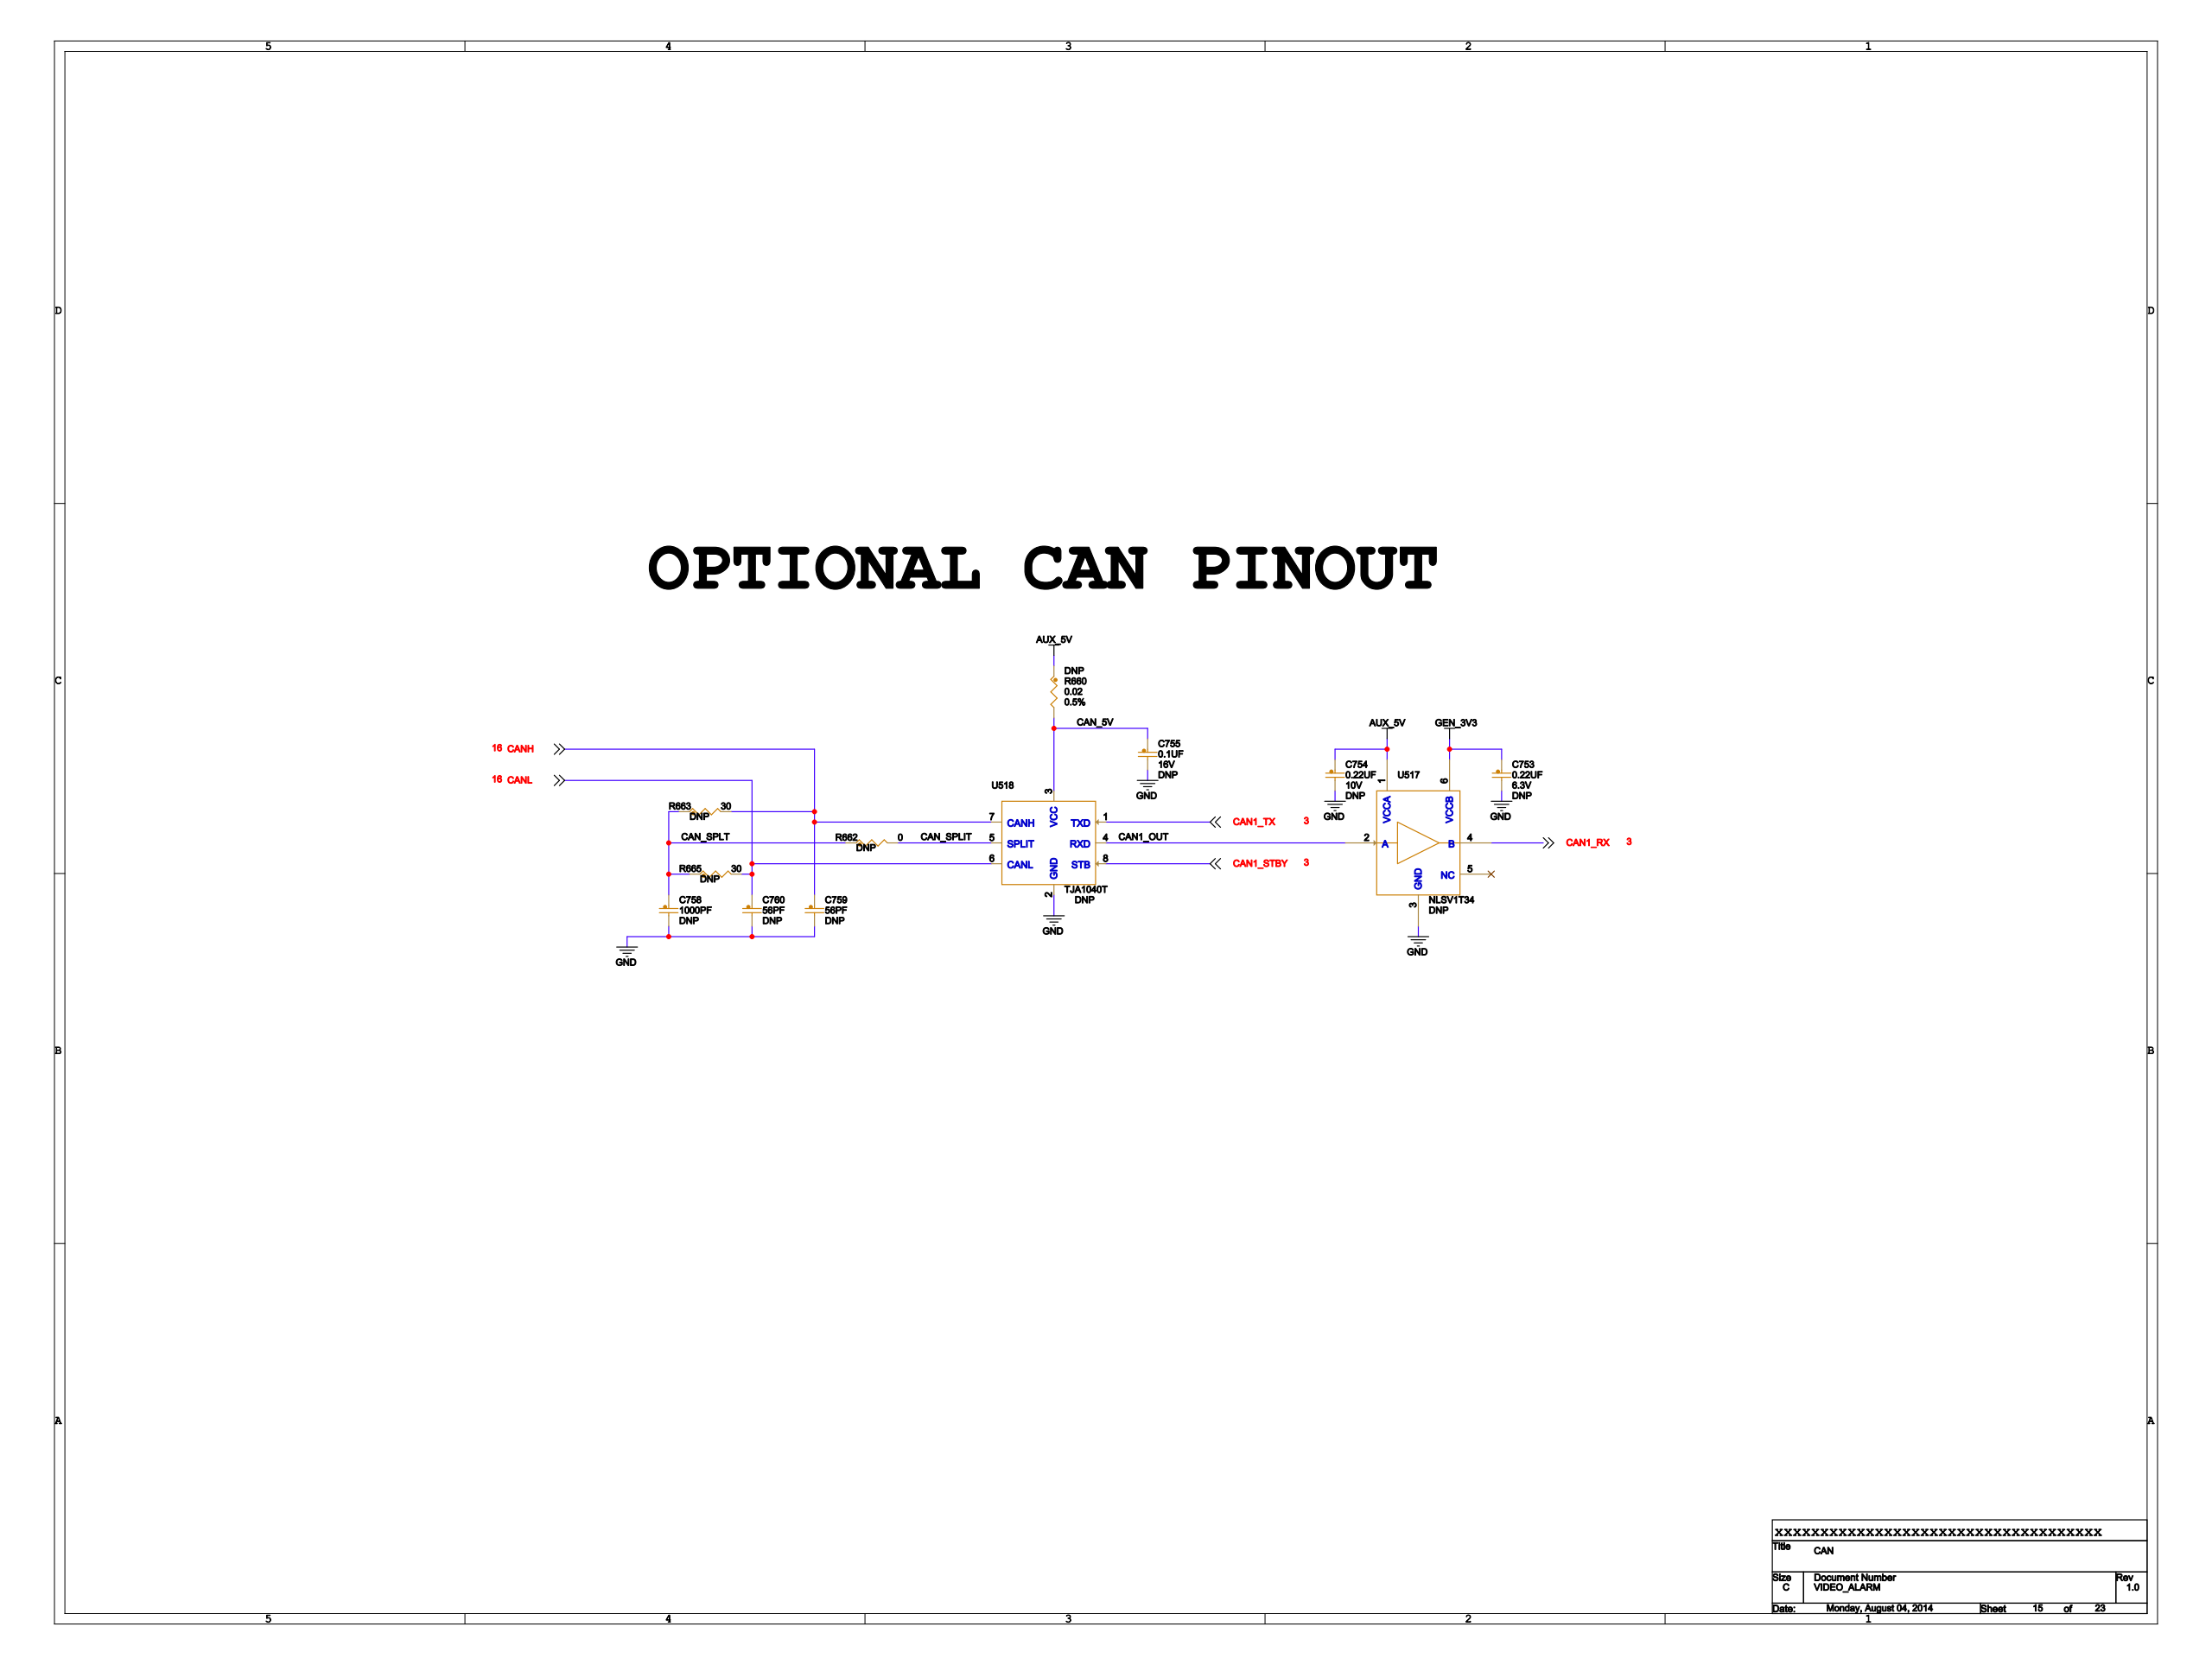Circuit board | Cadence Allegro | 994 parts | 728 nets | one sheet of the schematic
Parts on this sheet (reference | value | footprint):
C753 | 0.22UF | 0603_CC
C754 | 0.22UF | 0603_CC
C755 | 0.1UF | 0603_CC
C758 | 1000PF | 0603_CC
C759 | 56PF | 0603_CC
C760 | 56PF | 0603_CC
R660 | 0.02 | 0805_CC
R662 | 0 | 0603_CC
R663 | 30 | 0603_CC
R665 | 30 | 0603_CC
U517 | NLSV1T34 | ULLGA6_1P45X1_0P5MM
U518 | TJA1040T | SO8_1P27_4X5
Nets of these parts (net: part-pin ...):
GND: C753-2 C754-2 C755-2 C758-2 C759-2 C760-2 U517-3 U518-2
GEN_3V3: C753-1 U517-6
CANL: C760-1 R665-2 U518-6
CANH: C759-1 R663-2 U518-7
CAN_SPLT: C758-1 R662-1 R663-1 R665-1
CAN_SPLIT: R662-2 U518-5
AUX_5V: C754-1 R660-1 U517-1
CAN_5V: C755-1 R660-2 U518-3
CAN1_OUT: U517-2 U518-4
CAN1_STBY: U518-8
CAN1_TX: U518-1
CAN1_RX: U517-4